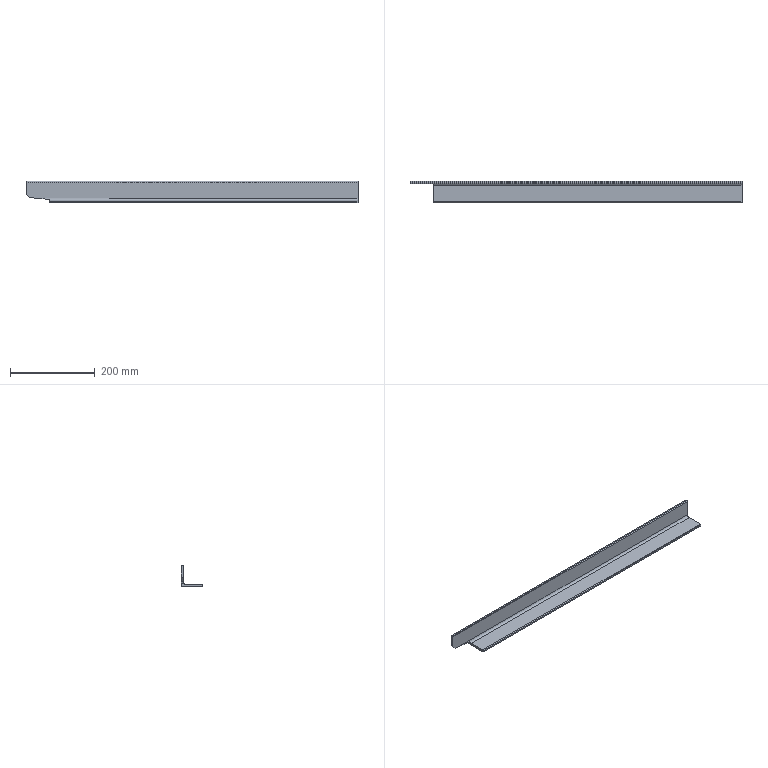Part | SolidWorks | 1 solid | 15 faces | box 783.5 x 50 x 50 mm | volume 360247 mm3 | plane 12 | cylinder 3 | commonest cylinder face diameters 3.333 x2 11 x1
STEP:
#1=CARTESIAN_POINT('',(-335.25,-50.,0.));
#2=VERTEX_POINT('',#1);
#3=CARTESIAN_POINT('',(391.75,-50.,0.));
#4=VERTEX_POINT('',#3);
#5=CARTESIAN_POINT('',(-391.75,-50.,0.));
#6=DIRECTION('',(1.,0.,0.));
#7=VECTOR('',#6,1000.);
#8=LINE('',#5,#7);
#9=EDGE_CURVE('',#2,#4,#8,.T.);
#10=ORIENTED_EDGE('',*,*,#9,.F.);
#11=CARTESIAN_POINT('',(-335.25,0.,0.));
#12=VERTEX_POINT('',#11);
#13=CARTESIAN_POINT('',(-335.25,-50.,0.));
#14=DIRECTION('',(0.,1.,0.));
#15=VECTOR('',#14,1000.);
#16=LINE('',#13,#15);
#17=EDGE_CURVE('',#2,#12,#16,.T.);
#18=ORIENTED_EDGE('',*,*,#17,.T.);
#19=CARTESIAN_POINT('',(391.75,0.,0.));
#20=VERTEX_POINT('',#19);
#21=CARTESIAN_POINT('',(-391.75,0.,0.));
#22=DIRECTION('',(1.,0.,0.));
#23=VECTOR('',#22,1000.);
#24=LINE('',#21,#23);
#25=EDGE_CURVE('',#12,#20,#24,.T.);
#26=ORIENTED_EDGE('',*,*,#25,.T.);
#27=CARTESIAN_POINT('',(391.75,-50.,0.));
#28=DIRECTION('',(0.,-1.,0.));
#29=VECTOR('',#28,1000.);
#30=LINE('',#27,#29);
#31=EDGE_CURVE('',#20,#4,#30,.T.);
#32=ORIENTED_EDGE('',*,*,#31,.T.);
#33=EDGE_LOOP('',(#10,#18,#26,#32));
#34=FACE_OUTER_BOUND('',#33,.T.);
#35=CARTESIAN_POINT('',(-391.75,-50.,0.));
#36=DIRECTION('',(0.,0.,1.));
#37=DIRECTION('',(1.,0.,0.));
#38=AXIS2_PLACEMENT_3D('',#35,#36,#37);
#39=PLANE('',#38);
#40=ADVANCED_FACE('',(#34),#39,.F.);
#41=CARTESIAN_POINT('',(-335.25,-50.,3.333));
#42=VERTEX_POINT('',#41);
#43=CARTESIAN_POINT('',(391.75,-50.,3.333));
#44=VERTEX_POINT('',#43);
#45=CARTESIAN_POINT('',(-391.75,-50.,3.333));
#46=DIRECTION('',(1.,0.,0.));
#47=VECTOR('',#46,1000.);
#48=LINE('',#45,#47);
#49=EDGE_CURVE('',#42,#44,#48,.T.);
#50=ORIENTED_EDGE('',*,*,#49,.F.);
#51=CARTESIAN_POINT('',(-335.25,-50.,-7.499));
#52=DIRECTION('',(0.,0.,-1.));
#53=VECTOR('',#52,1000.);
#54=LINE('',#51,#53);
#55=EDGE_CURVE('',#42,#2,#54,.T.);
#56=ORIENTED_EDGE('',*,*,#55,.T.);
#57=ORIENTED_EDGE('',*,*,#9,.T.);
#58=CARTESIAN_POINT('',(391.75,-50.,0.));
#59=DIRECTION('',(0.,0.,1.));
#60=VECTOR('',#59,1000.);
#61=LINE('',#58,#60);
#62=EDGE_CURVE('',#4,#44,#61,.T.);
#63=ORIENTED_EDGE('',*,*,#62,.T.);
#64=EDGE_LOOP('',(#50,#56,#57,#63));
#65=FACE_OUTER_BOUND('',#64,.T.);
#66=CARTESIAN_POINT('',(-391.75,-50.,0.));
#67=DIRECTION('',(0.,1.,0.));
#68=DIRECTION('',(-1.,0.,0.));
#69=AXIS2_PLACEMENT_3D('',#66,#67,#68);
#70=PLANE('',#69);
#71=ADVANCED_FACE('',(#65),#70,.F.);
#72=CARTESIAN_POINT('',(-335.25,-48.333,5.));
#73=VERTEX_POINT('',#72);
#74=CARTESIAN_POINT('',(391.75,-48.333,5.));
#75=VERTEX_POINT('',#74);
#76=CARTESIAN_POINT('',(-391.75,-48.333,5.));
#77=DIRECTION('',(1.,0.,0.));
#78=VECTOR('',#77,1000.);
#79=LINE('',#76,#78);
#80=EDGE_CURVE('',#73,#75,#79,.T.);
#81=ORIENTED_EDGE('',*,*,#80,.F.);
#82=CARTESIAN_POINT('',(-335.25,-48.333,3.333));
#83=DIRECTION('',(1.,0.,0.));
#84=DIRECTION('',(0.,0.,-1.));
#85=AXIS2_PLACEMENT_3D('',#82,#83,#84);
#86=CIRCLE('',#85,1.667);
#87=EDGE_CURVE('',#73,#42,#86,.T.);
#88=ORIENTED_EDGE('',*,*,#87,.T.);
#89=ORIENTED_EDGE('',*,*,#49,.T.);
#90=CARTESIAN_POINT('',(391.75,-48.333,3.333));
#91=DIRECTION('',(-1.,0.,0.));
#92=DIRECTION('',(0.,-1.,0.));
#93=AXIS2_PLACEMENT_3D('',#90,#91,#92);
#94=CIRCLE('',#93,1.667);
#95=EDGE_CURVE('',#44,#75,#94,.T.);
#96=ORIENTED_EDGE('',*,*,#95,.T.);
#97=EDGE_LOOP('',(#81,#88,#89,#96));
#98=FACE_OUTER_BOUND('',#97,.T.);
#99=CARTESIAN_POINT('',(-391.75,-48.333,3.333));
#100=DIRECTION('',(1.,0.,0.));
#101=DIRECTION('',(0.,1.,0.));
#102=AXIS2_PLACEMENT_3D('',#99,#100,#101);
#103=CYLINDRICAL_SURFACE('',#102,1.667);
#104=ADVANCED_FACE('',(#98),#103,.T.);
#105=CARTESIAN_POINT('',(-335.25,-10.5,5.));
#106=VERTEX_POINT('',#105);
#107=CARTESIAN_POINT('',(391.75,-10.5,5.));
#108=VERTEX_POINT('',#107);
#109=CARTESIAN_POINT('',(-391.75,-10.5,5.));
#110=DIRECTION('',(1.,0.,0.));
#111=VECTOR('',#110,1000.);
#112=LINE('',#109,#111);
#113=EDGE_CURVE('',#106,#108,#112,.T.);
#114=ORIENTED_EDGE('',*,*,#113,.F.);
#115=CARTESIAN_POINT('',(-335.25,-10.5,5.));
#116=DIRECTION('',(0.,-1.,0.));
#117=VECTOR('',#116,1000.);
#118=LINE('',#115,#117);
#119=EDGE_CURVE('',#106,#73,#118,.T.);
#120=ORIENTED_EDGE('',*,*,#119,.T.);
#121=ORIENTED_EDGE('',*,*,#80,.T.);
#122=CARTESIAN_POINT('',(391.75,-10.5,5.));
#123=DIRECTION('',(0.,1.,0.));
#124=VECTOR('',#123,1000.);
#125=LINE('',#122,#124);
#126=EDGE_CURVE('',#75,#108,#125,.T.);
#127=ORIENTED_EDGE('',*,*,#126,.T.);
#128=EDGE_LOOP('',(#114,#120,#121,#127));
#129=FACE_OUTER_BOUND('',#128,.T.);
#130=CARTESIAN_POINT('',(-391.75,-10.5,5.));
#131=DIRECTION('',(0.,0.,-1.));
#132=DIRECTION('',(0.,1.,0.));
#133=AXIS2_PLACEMENT_3D('',#130,#131,#132);
#134=PLANE('',#133);
#135=ADVANCED_FACE('',(#129),#134,.F.);
#136=CARTESIAN_POINT('',(-339.727,-5.889,7.501));
#137=VERTEX_POINT('',#136);
#138=CARTESIAN_POINT('',(-335.25,-5.889,7.501));
#139=VERTEX_POINT('',#138);
#140=CARTESIAN_POINT('',(-391.75,-5.889,7.501));
#141=DIRECTION('',(1.,0.,0.));
#142=VECTOR('',#141,1000.);
#143=LINE('',#140,#142);
#144=EDGE_CURVE('',#137,#139,#143,.T.);
#145=ORIENTED_EDGE('',*,*,#144,.T.);
#146=CARTESIAN_POINT('',(-335.25,-10.5,10.5));
#147=DIRECTION('',(-1.,0.,0.));
#148=DIRECTION('',(0.,0.,-1.));
#149=AXIS2_PLACEMENT_3D('',#146,#147,#148);
#150=CIRCLE('',#149,5.5);
#151=EDGE_CURVE('',#139,#106,#150,.T.);
#152=ORIENTED_EDGE('',*,*,#151,.T.);
#153=ORIENTED_EDGE('',*,*,#113,.T.);
#154=CARTESIAN_POINT('',(391.75,-5.,10.5));
#155=VERTEX_POINT('',#154);
#156=CARTESIAN_POINT('',(391.75,-10.5,10.5));
#157=DIRECTION('',(1.,0.,0.));
#158=DIRECTION('',(0.,1.,0.));
#159=AXIS2_PLACEMENT_3D('',#156,#157,#158);
#160=CIRCLE('',#159,5.5);
#161=EDGE_CURVE('',#108,#155,#160,.T.);
#162=ORIENTED_EDGE('',*,*,#161,.T.);
#163=CARTESIAN_POINT('',(-368.257,-5.,10.5));
#164=VERTEX_POINT('',#163);
#165=CARTESIAN_POINT('',(-391.75,-5.,10.5));
#166=DIRECTION('',(1.,0.,0.));
#167=VECTOR('',#166,1000.);
#168=LINE('',#165,#167);
#169=EDGE_CURVE('',#164,#155,#168,.T.);
#170=ORIENTED_EDGE('',*,*,#169,.F.);
#171=CARTESIAN_POINT('',(-368.257,-5.,10.5));
#172=CARTESIAN_POINT('',(-358.057,-5.,9.428));
#173=CARTESIAN_POINT('',(-348.278,-5.305,8.4));
#174=CARTESIAN_POINT('',(-339.727,-5.889,7.501));
#175=(BOUNDED_CURVE()B_SPLINE_CURVE(3,(#171,#172,#173,#174),.UNSPECIFIED.,.F.,.T.)B_SPLINE_CURVE_WITH_KNOTS((4,4),(4.712,5.289),.UNSPECIFIED.)CURVE()GEOMETRIC_REPRESENTATION_ITEM()RATIONAL_B_SPLINE_CURVE((1.,0.9725,0.9725,1.))REPRESENTATION_ITEM(''));
#176=EDGE_CURVE('',#164,#137,#175,.T.);
#177=ORIENTED_EDGE('',*,*,#176,.T.);
#178=EDGE_LOOP('',(#145,#152,#153,#162,#170,#177));
#179=FACE_OUTER_BOUND('',#178,.T.);
#180=CARTESIAN_POINT('',(-391.75,-10.5,10.5));
#181=DIRECTION('',(1.,0.,0.));
#182=DIRECTION('',(0.,1.,0.));
#183=AXIS2_PLACEMENT_3D('',#180,#181,#182);
#184=CYLINDRICAL_SURFACE('',#183,5.5);
#185=ADVANCED_FACE('',(#179),#184,.F.);
#186=CARTESIAN_POINT('',(-391.75,-5.,21.973));
#187=VERTEX_POINT('',#186);
#188=CARTESIAN_POINT('',(-382.795,-5.,12.028));
#189=VERTEX_POINT('',#188);
#190=CARTESIAN_POINT('',(-404.858,-5.,36.531));
#191=DIRECTION('',(0.6691,0.,-0.7431));
#192=VECTOR('',#191,1000.);
#193=LINE('',#190,#192);
#194=EDGE_CURVE('',#187,#189,#193,.T.);
#195=ORIENTED_EDGE('',*,*,#194,.T.);
#196=CARTESIAN_POINT('',(-395.426,-5.,13.356));
#197=DIRECTION('',(0.9945,0.,-0.1045));
#198=VECTOR('',#197,1000.);
#199=LINE('',#196,#198);
#200=EDGE_CURVE('',#189,#164,#199,.T.);
#201=ORIENTED_EDGE('',*,*,#200,.T.);
#202=ORIENTED_EDGE('',*,*,#169,.T.);
#203=CARTESIAN_POINT('',(391.75,-5.,48.333));
#204=VERTEX_POINT('',#203);
#205=CARTESIAN_POINT('',(391.75,-5.,48.333));
#206=DIRECTION('',(0.,0.,1.));
#207=VECTOR('',#206,1000.);
#208=LINE('',#205,#207);
#209=EDGE_CURVE('',#155,#204,#208,.T.);
#210=ORIENTED_EDGE('',*,*,#209,.T.);
#211=CARTESIAN_POINT('',(-391.75,-5.,48.333));
#212=VERTEX_POINT('',#211);
#213=CARTESIAN_POINT('',(-391.75,-5.,48.333));
#214=DIRECTION('',(1.,0.,0.));
#215=VECTOR('',#214,1000.);
#216=LINE('',#213,#215);
#217=EDGE_CURVE('',#212,#204,#216,.T.);
#218=ORIENTED_EDGE('',*,*,#217,.F.);
#219=CARTESIAN_POINT('',(-391.75,-5.,48.333));
#220=DIRECTION('',(0.,0.,1.));
#221=VECTOR('',#220,1000.);
#222=LINE('',#219,#221);
#223=EDGE_CURVE('',#187,#212,#222,.T.);
#224=ORIENTED_EDGE('',*,*,#223,.F.);
#225=EDGE_LOOP('',(#195,#201,#202,#210,#218,#224));
#226=FACE_OUTER_BOUND('',#225,.T.);
#227=CARTESIAN_POINT('',(-391.75,-5.,48.333));
#228=DIRECTION('',(0.,1.,0.));
#229=DIRECTION('',(-1.,0.,0.));
#230=AXIS2_PLACEMENT_3D('',#227,#228,#229);
#231=PLANE('',#230);
#232=ADVANCED_FACE('',(#226),#231,.F.);
#233=CARTESIAN_POINT('',(391.75,-3.333,50.));
#234=VERTEX_POINT('',#233);
#235=CARTESIAN_POINT('',(391.75,-3.333,48.333));
#236=DIRECTION('',(-1.,0.,0.));
#237=DIRECTION('',(0.,1.,0.));
#238=AXIS2_PLACEMENT_3D('',#235,#236,#237);
#239=CIRCLE('',#238,1.667);
#240=EDGE_CURVE('',#204,#234,#239,.T.);
#241=ORIENTED_EDGE('',*,*,#240,.T.);
#242=CARTESIAN_POINT('',(-391.75,-3.333,50.));
#243=VERTEX_POINT('',#242);
#244=CARTESIAN_POINT('',(-391.75,-3.333,50.));
#245=DIRECTION('',(1.,0.,0.));
#246=VECTOR('',#245,1000.);
#247=LINE('',#244,#246);
#248=EDGE_CURVE('',#243,#234,#247,.T.);
#249=ORIENTED_EDGE('',*,*,#248,.F.);
#250=CARTESIAN_POINT('',(-391.75,-3.333,48.333));
#251=DIRECTION('',(-1.,0.,0.));
#252=DIRECTION('',(0.,1.,0.));
#253=AXIS2_PLACEMENT_3D('',#250,#251,#252);
#254=CIRCLE('',#253,1.667);
#255=EDGE_CURVE('',#212,#243,#254,.T.);
#256=ORIENTED_EDGE('',*,*,#255,.F.);
#257=ORIENTED_EDGE('',*,*,#217,.T.);
#258=EDGE_LOOP('',(#241,#249,#256,#257));
#259=FACE_OUTER_BOUND('',#258,.T.);
#260=CARTESIAN_POINT('',(-391.75,-3.333,48.333));
#261=DIRECTION('',(1.,0.,0.));
#262=DIRECTION('',(0.,1.,0.));
#263=AXIS2_PLACEMENT_3D('',#260,#261,#262);
#264=CYLINDRICAL_SURFACE('',#263,1.667);
#265=ADVANCED_FACE('',(#259),#264,.T.);
#266=CARTESIAN_POINT('',(391.75,0.,50.));
#267=VERTEX_POINT('',#266);
#268=CARTESIAN_POINT('',(391.75,0.,50.));
#269=DIRECTION('',(0.,1.,0.));
#270=VECTOR('',#269,1000.);
#271=LINE('',#268,#270);
#272=EDGE_CURVE('',#234,#267,#271,.T.);
#273=ORIENTED_EDGE('',*,*,#272,.T.);
#274=CARTESIAN_POINT('',(-391.75,0.,50.));
#275=VERTEX_POINT('',#274);
#276=CARTESIAN_POINT('',(-391.75,0.,50.));
#277=DIRECTION('',(1.,0.,0.));
#278=VECTOR('',#277,1000.);
#279=LINE('',#276,#278);
#280=EDGE_CURVE('',#275,#267,#279,.T.);
#281=ORIENTED_EDGE('',*,*,#280,.F.);
#282=CARTESIAN_POINT('',(-391.75,0.,50.));
#283=DIRECTION('',(0.,1.,0.));
#284=VECTOR('',#283,1000.);
#285=LINE('',#282,#284);
#286=EDGE_CURVE('',#243,#275,#285,.T.);
#287=ORIENTED_EDGE('',*,*,#286,.F.);
#288=ORIENTED_EDGE('',*,*,#248,.T.);
#289=EDGE_LOOP('',(#273,#281,#287,#288));
#290=FACE_OUTER_BOUND('',#289,.T.);
#291=CARTESIAN_POINT('',(-391.75,0.,50.));
#292=DIRECTION('',(0.,0.,-1.));
#293=DIRECTION('',(0.,1.,0.));
#294=AXIS2_PLACEMENT_3D('',#291,#292,#293);
#295=PLANE('',#294);
#296=ADVANCED_FACE('',(#290),#295,.F.);
#297=ORIENTED_EDGE('',*,*,#25,.F.);
#298=CARTESIAN_POINT('',(-335.25,0.,7.501));
#299=VERTEX_POINT('',#298);
#300=CARTESIAN_POINT('',(-335.25,0.,0.));
#301=DIRECTION('',(0.,0.,-1.));
#302=VECTOR('',#301,1000.);
#303=LINE('',#300,#302);
#304=EDGE_CURVE('',#299,#12,#303,.T.);
#305=ORIENTED_EDGE('',*,*,#304,.F.);
#306=CARTESIAN_POINT('',(-339.727,0.,7.501));
#307=VERTEX_POINT('',#306);
#308=CARTESIAN_POINT('',(-335.25,0.,7.501));
#309=DIRECTION('',(1.,0.,0.));
#310=VECTOR('',#309,1000.);
#311=LINE('',#308,#310);
#312=EDGE_CURVE('',#307,#299,#311,.T.);
#313=ORIENTED_EDGE('',*,*,#312,.F.);
#314=CARTESIAN_POINT('',(-382.795,0.,12.028));
#315=VERTEX_POINT('',#314);
#316=CARTESIAN_POINT('',(-339.727,0.,7.501));
#317=DIRECTION('',(0.9945,0.,-0.1045));
#318=VECTOR('',#317,1000.);
#319=LINE('',#316,#318);
#320=EDGE_CURVE('',#315,#307,#319,.T.);
#321=ORIENTED_EDGE('',*,*,#320,.F.);
#322=CARTESIAN_POINT('',(-391.75,0.,21.973));
#323=VERTEX_POINT('',#322);
#324=CARTESIAN_POINT('',(-382.795,0.,12.028));
#325=DIRECTION('',(0.6691,0.,-0.7431));
#326=VECTOR('',#325,1000.);
#327=LINE('',#324,#326);
#328=EDGE_CURVE('',#323,#315,#327,.T.);
#329=ORIENTED_EDGE('',*,*,#328,.F.);
#330=CARTESIAN_POINT('',(-391.75,0.,0.));
#331=DIRECTION('',(0.,0.,-1.));
#332=VECTOR('',#331,1000.);
#333=LINE('',#330,#332);
#334=EDGE_CURVE('',#275,#323,#333,.T.);
#335=ORIENTED_EDGE('',*,*,#334,.F.);
#336=ORIENTED_EDGE('',*,*,#280,.T.);
#337=CARTESIAN_POINT('',(391.75,0.,0.));
#338=DIRECTION('',(0.,0.,-1.));
#339=VECTOR('',#338,1000.);
#340=LINE('',#337,#339);
#341=EDGE_CURVE('',#267,#20,#340,.T.);
#342=ORIENTED_EDGE('',*,*,#341,.T.);
#343=EDGE_LOOP('',(#297,#305,#313,#321,#329,#335,#336,#342));
#344=FACE_OUTER_BOUND('',#343,.T.);
#345=CARTESIAN_POINT('',(-391.75,0.,0.));
#346=DIRECTION('',(0.,-1.,0.));
#347=DIRECTION('',(1.,0.,0.));
#348=AXIS2_PLACEMENT_3D('',#345,#346,#347);
#349=PLANE('',#348);
#350=ADVANCED_FACE('',(#344),#349,.F.);
#351=ORIENTED_EDGE('',*,*,#334,.T.);
#352=CARTESIAN_POINT('',(-391.75,-3.333,21.973));
#353=DIRECTION('',(0.,-1.,0.));
#354=VECTOR('',#353,1000.);
#355=LINE('',#352,#354);
#356=EDGE_CURVE('',#323,#187,#355,.T.);
#357=ORIENTED_EDGE('',*,*,#356,.T.);
#358=ORIENTED_EDGE('',*,*,#223,.T.);
#359=ORIENTED_EDGE('',*,*,#255,.T.);
#360=ORIENTED_EDGE('',*,*,#286,.T.);
#361=EDGE_LOOP('',(#351,#357,#358,#359,#360));
#362=FACE_OUTER_BOUND('',#361,.T.);
#363=CARTESIAN_POINT('',(-391.75,-3.333,48.333));
#364=DIRECTION('',(1.,0.,0.));
#365=DIRECTION('',(0.,1.,0.));
#366=AXIS2_PLACEMENT_3D('',#363,#364,#365);
#367=PLANE('',#366);
#368=ADVANCED_FACE('',(#362),#367,.F.);
#369=ORIENTED_EDGE('',*,*,#31,.F.);
#370=ORIENTED_EDGE('',*,*,#341,.F.);
#371=ORIENTED_EDGE('',*,*,#272,.F.);
#372=ORIENTED_EDGE('',*,*,#240,.F.);
#373=ORIENTED_EDGE('',*,*,#209,.F.);
#374=ORIENTED_EDGE('',*,*,#161,.F.);
#375=ORIENTED_EDGE('',*,*,#126,.F.);
#376=ORIENTED_EDGE('',*,*,#95,.F.);
#377=ORIENTED_EDGE('',*,*,#62,.F.);
#378=EDGE_LOOP('',(#369,#370,#371,#372,#373,#374,#375,#376,#377));
#379=FACE_OUTER_BOUND('',#378,.T.);
#380=CARTESIAN_POINT('',(391.75,-3.333,48.333));
#381=DIRECTION('',(1.,0.,0.));
#382=DIRECTION('',(0.,1.,0.));
#383=AXIS2_PLACEMENT_3D('',#380,#381,#382);
#384=PLANE('',#383);
#385=ADVANCED_FACE('',(#379),#384,.T.);
#386=ORIENTED_EDGE('',*,*,#55,.F.);
#387=ORIENTED_EDGE('',*,*,#87,.F.);
#388=ORIENTED_EDGE('',*,*,#119,.F.);
#389=ORIENTED_EDGE('',*,*,#151,.F.);
#390=CARTESIAN_POINT('',(-335.25,-50.,7.501));
#391=DIRECTION('',(0.,1.,0.));
#392=VECTOR('',#391,1000.);
#393=LINE('',#390,#392);
#394=EDGE_CURVE('',#139,#299,#393,.T.);
#395=ORIENTED_EDGE('',*,*,#394,.T.);
#396=ORIENTED_EDGE('',*,*,#304,.T.);
#397=ORIENTED_EDGE('',*,*,#17,.F.);
#398=EDGE_LOOP('',(#386,#387,#388,#389,#395,#396,#397));
#399=FACE_OUTER_BOUND('',#398,.T.);
#400=CARTESIAN_POINT('',(-335.25,-50.,0.));
#401=DIRECTION('',(1.,0.,0.));
#402=DIRECTION('',(0.,0.,-1.));
#403=AXIS2_PLACEMENT_3D('',#400,#401,#402);
#404=PLANE('',#403);
#405=ADVANCED_FACE('',(#399),#404,.F.);
#406=CARTESIAN_POINT('',(-339.727,-50.,7.501));
#407=DIRECTION('',(0.,1.,0.));
#408=VECTOR('',#407,1000.);
#409=LINE('',#406,#408);
#410=EDGE_CURVE('',#137,#307,#409,.T.);
#411=ORIENTED_EDGE('',*,*,#410,.T.);
#412=ORIENTED_EDGE('',*,*,#312,.T.);
#413=ORIENTED_EDGE('',*,*,#394,.F.);
#414=ORIENTED_EDGE('',*,*,#144,.F.);
#415=EDGE_LOOP('',(#411,#412,#413,#414));
#416=FACE_OUTER_BOUND('',#415,.T.);
#417=CARTESIAN_POINT('',(-335.25,-50.,7.501));
#418=DIRECTION('',(0.,0.,1.));
#419=DIRECTION('',(1.,0.,0.));
#420=AXIS2_PLACEMENT_3D('',#417,#418,#419);
#421=PLANE('',#420);
#422=ADVANCED_FACE('',(#416),#421,.F.);
#423=ORIENTED_EDGE('',*,*,#200,.F.);
#424=CARTESIAN_POINT('',(-382.795,-50.,12.028));
#425=DIRECTION('',(0.,1.,0.));
#426=VECTOR('',#425,1000.);
#427=LINE('',#424,#426);
#428=EDGE_CURVE('',#189,#315,#427,.T.);
#429=ORIENTED_EDGE('',*,*,#428,.T.);
#430=ORIENTED_EDGE('',*,*,#320,.T.);
#431=ORIENTED_EDGE('',*,*,#410,.F.);
#432=ORIENTED_EDGE('',*,*,#176,.F.);
#433=EDGE_LOOP('',(#423,#429,#430,#431,#432));
#434=FACE_OUTER_BOUND('',#433,.T.);
#435=CARTESIAN_POINT('',(-339.727,-50.,7.501));
#436=DIRECTION('',(0.1045,0.,0.9945));
#437=DIRECTION('',(0.9945,0.,-0.1045));
#438=AXIS2_PLACEMENT_3D('',#435,#436,#437);
#439=PLANE('',#438);
#440=ADVANCED_FACE('',(#434),#439,.F.);
#441=ORIENTED_EDGE('',*,*,#356,.F.);
#442=ORIENTED_EDGE('',*,*,#328,.T.);
#443=ORIENTED_EDGE('',*,*,#428,.F.);
#444=ORIENTED_EDGE('',*,*,#194,.F.);
#445=EDGE_LOOP('',(#441,#442,#443,#444));
#446=FACE_OUTER_BOUND('',#445,.T.);
#447=CARTESIAN_POINT('',(-382.795,-50.,12.028));
#448=DIRECTION('',(0.7431,0.,0.6691));
#449=DIRECTION('',(0.6691,0.,-0.7431));
#450=AXIS2_PLACEMENT_3D('',#447,#448,#449);
#451=PLANE('',#450);
#452=ADVANCED_FACE('',(#446),#451,.F.);
#453=CLOSED_SHELL('',(#40,#71,#104,#135,#185,#232,#265,#296,#350,#368,#385,#405,#422,#440,#452));
#454=MANIFOLD_SOLID_BREP('',#453);
#455=CARTESIAN_POINT('',(0.,0.,0.));
#456=DIRECTION('',(0.,0.,1.));
#457=DIRECTION('',(1.,0.,0.));
#458=AXIS2_PLACEMENT_3D('',#455,#456,#457);
#459=(LENGTH_UNIT()NAMED_UNIT(*)SI_UNIT(.MILLI.,.METRE.));
#460=UNCERTAINTY_MEASURE_WITH_UNIT(LENGTH_MEASURE(0.00001),#459,'','');
#461=(NAMED_UNIT(*)PLANE_ANGLE_UNIT()SI_UNIT($,.RADIAN.));
#462=(NAMED_UNIT(*)SI_UNIT($,.STERADIAN.)SOLID_ANGLE_UNIT());
#463=(GEOMETRIC_REPRESENTATION_CONTEXT(3)GLOBAL_UNCERTAINTY_ASSIGNED_CONTEXT((#460))GLOBAL_UNIT_ASSIGNED_CONTEXT((#459,#461,#462))REPRESENTATION_CONTEXT('',''));
#464=ADVANCED_BREP_SHAPE_REPRESENTATION('',(#454,#458),#463);